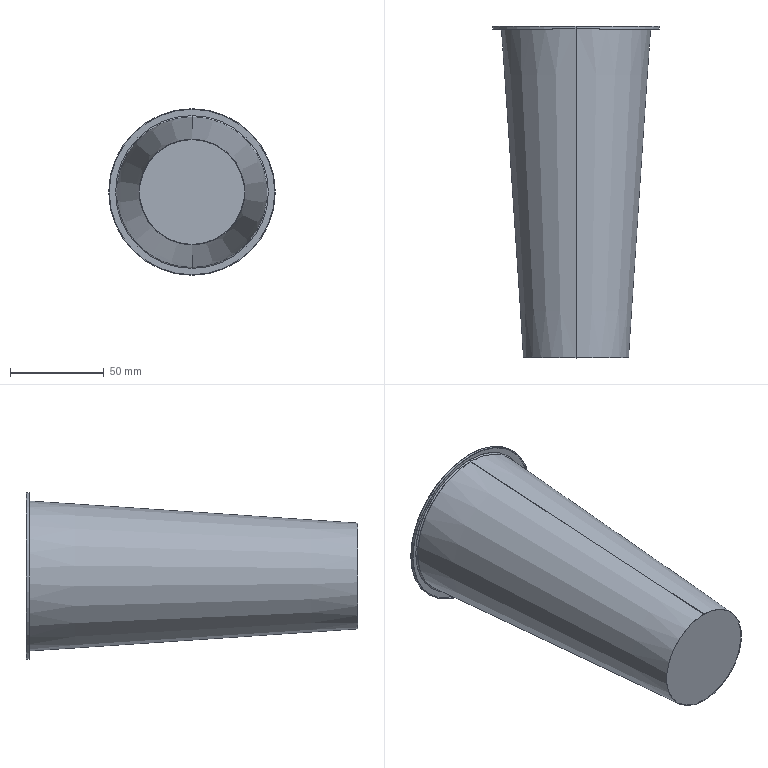Part | SolidWorks | features RefAxis 1, Revolution 1 | 1 solid | 19 faces | box 89 x 177.3 x 89 mm | volume 12581 mm3 | torus 6 | plane 5 | cone 4 | cylinder 4 | commonest cylinder face diameters 88.4 x2 89 x2
STEP:
#1=CARTESIAN_POINT('',(0.,-0.3,28.281));
#2=VERTEX_POINT('',#1);
#3=CARTESIAN_POINT('',(0.,-0.3,-28.281));
#4=VERTEX_POINT('',#3);
#5=CARTESIAN_POINT('',(0.,-0.3,0.));
#6=DIRECTION('',(0.,1.,0.));
#7=DIRECTION('',(0.,0.,1.));
#8=AXIS2_PLACEMENT_3D('',#5,#6,#7);
#9=CIRCLE('',#8,28.281);
#10=EDGE_CURVE('',#2,#4,#9,.T.);
#11=ORIENTED_EDGE('',*,*,#10,.T.);
#12=CARTESIAN_POINT('',(0.,176.047,-40.137));
#13=VERTEX_POINT('',#12);
#14=CARTESIAN_POINT('',(0.,176.047,-40.137));
#15=DIRECTION('',(0.,0.9977,-0.06708));
#16=VECTOR('',#15,1000.);
#17=LINE('',#14,#16);
#18=EDGE_CURVE('',#4,#13,#17,.T.);
#19=ORIENTED_EDGE('',*,*,#18,.T.);
#20=CARTESIAN_POINT('',(0.,176.047,40.137));
#21=VERTEX_POINT('',#20);
#22=CARTESIAN_POINT('',(0.,176.047,0.));
#23=DIRECTION('',(0.,1.,0.));
#24=DIRECTION('',(0.,0.,1.));
#25=AXIS2_PLACEMENT_3D('',#22,#23,#24);
#26=CIRCLE('',#25,40.137);
#27=EDGE_CURVE('',#21,#13,#26,.T.);
#28=ORIENTED_EDGE('',*,*,#27,.F.);
#29=CARTESIAN_POINT('',(0.,176.047,40.137));
#30=DIRECTION('',(0.,0.9977,0.06708));
#31=VECTOR('',#30,1000.);
#32=LINE('',#29,#31);
#33=EDGE_CURVE('',#2,#21,#32,.T.);
#34=ORIENTED_EDGE('',*,*,#33,.F.);
#35=EDGE_LOOP('',(#11,#19,#28,#34));
#36=FACE_OUTER_BOUND('',#35,.T.);
#37=CARTESIAN_POINT('',(0.,176.047,0.));
#38=DIRECTION('',(0.,1.,0.));
#39=DIRECTION('',(0.,0.,1.));
#40=AXIS2_PLACEMENT_3D('',#37,#38,#39);
#41=CONICAL_SURFACE('',#40,40.137,0.06713);
#42=ADVANCED_FACE('',(#36),#41,.T.);
#43=CARTESIAN_POINT('',(0.,176.7,-40.835));
#44=VERTEX_POINT('',#43);
#45=CARTESIAN_POINT('',(0.,176.7,40.835));
#46=VERTEX_POINT('',#45);
#47=CARTESIAN_POINT('',(0.,176.7,0.));
#48=DIRECTION('',(0.,1.,0.));
#49=DIRECTION('',(0.,0.,1.));
#50=AXIS2_PLACEMENT_3D('',#47,#48,#49);
#51=CIRCLE('',#50,40.835);
#52=EDGE_CURVE('',#44,#46,#51,.T.);
#53=ORIENTED_EDGE('',*,*,#52,.F.);
#54=CARTESIAN_POINT('',(0.,176.,-40.835));
#55=DIRECTION('',(1.,0.,0.));
#56=DIRECTION('',(0.,0.,-1.));
#57=AXIS2_PLACEMENT_3D('',#54,#55,#56);
#58=CIRCLE('',#57,0.7);
#59=EDGE_CURVE('',#44,#13,#58,.T.);
#60=ORIENTED_EDGE('',*,*,#59,.T.);
#61=CARTESIAN_POINT('',(0.,176.047,0.));
#62=DIRECTION('',(0.,1.,0.));
#63=DIRECTION('',(0.,0.,1.));
#64=AXIS2_PLACEMENT_3D('',#61,#62,#63);
#65=CIRCLE('',#64,40.137);
#66=EDGE_CURVE('',#13,#21,#65,.T.);
#67=ORIENTED_EDGE('',*,*,#66,.T.);
#68=CARTESIAN_POINT('',(0.,176.,40.835));
#69=DIRECTION('',(-1.,0.,0.));
#70=DIRECTION('',(0.,0.,1.));
#71=AXIS2_PLACEMENT_3D('',#68,#69,#70);
#72=CIRCLE('',#71,0.7);
#73=EDGE_CURVE('',#46,#21,#72,.T.);
#74=ORIENTED_EDGE('',*,*,#73,.F.);
#75=EDGE_LOOP('',(#53,#60,#67,#74));
#76=FACE_OUTER_BOUND('',#75,.T.);
#77=CARTESIAN_POINT('',(0.,176.,0.));
#78=DIRECTION('',(0.,1.,0.));
#79=DIRECTION('',(0.,0.,1.));
#80=AXIS2_PLACEMENT_3D('',#77,#78,#79);
#81=TOROIDAL_SURFACE('',#80,40.835,0.7);
#82=ADVANCED_FACE('',(#76),#81,.F.);
#83=CARTESIAN_POINT('',(0.,175.4,-44.2));
#84=VERTEX_POINT('',#83);
#85=CARTESIAN_POINT('',(0.,175.4,44.2));
#86=VERTEX_POINT('',#85);
#87=CARTESIAN_POINT('',(0.,175.4,0.));
#88=DIRECTION('',(0.,1.,0.));
#89=DIRECTION('',(0.,0.,1.));
#90=AXIS2_PLACEMENT_3D('',#87,#88,#89);
#91=CIRCLE('',#90,44.2);
#92=EDGE_CURVE('',#84,#86,#91,.T.);
#93=ORIENTED_EDGE('',*,*,#92,.F.);
#94=CARTESIAN_POINT('',(0.,176.7,-44.2));
#95=VERTEX_POINT('',#94);
#96=CARTESIAN_POINT('',(0.,0.,-44.2));
#97=DIRECTION('',(0.,1.,0.));
#98=VECTOR('',#97,1000.);
#99=LINE('',#96,#98);
#100=EDGE_CURVE('',#84,#95,#99,.T.);
#101=ORIENTED_EDGE('',*,*,#100,.T.);
#102=CARTESIAN_POINT('',(0.,176.7,44.2));
#103=VERTEX_POINT('',#102);
#104=CARTESIAN_POINT('',(0.,176.7,0.));
#105=DIRECTION('',(0.,1.,0.));
#106=DIRECTION('',(0.,0.,1.));
#107=AXIS2_PLACEMENT_3D('',#104,#105,#106);
#108=CIRCLE('',#107,44.2);
#109=EDGE_CURVE('',#95,#103,#108,.T.);
#110=ORIENTED_EDGE('',*,*,#109,.T.);
#111=CARTESIAN_POINT('',(0.,0.,44.2));
#112=DIRECTION('',(0.,1.,0.));
#113=VECTOR('',#112,1000.);
#114=LINE('',#111,#113);
#115=EDGE_CURVE('',#86,#103,#114,.T.);
#116=ORIENTED_EDGE('',*,*,#115,.F.);
#117=EDGE_LOOP('',(#93,#101,#110,#116));
#118=FACE_OUTER_BOUND('',#117,.T.);
#119=CARTESIAN_POINT('',(0.,0.,0.));
#120=DIRECTION('',(0.,1.,0.));
#121=DIRECTION('',(0.,0.,1.));
#122=AXIS2_PLACEMENT_3D('',#119,#120,#121);
#123=CYLINDRICAL_SURFACE('',#122,44.2);
#124=ADVANCED_FACE('',(#118),#123,.F.);
#125=CARTESIAN_POINT('',(0.,175.4,44.5));
#126=VERTEX_POINT('',#125);
#127=CARTESIAN_POINT('',(0.,175.4,-44.5));
#128=VERTEX_POINT('',#127);
#129=CARTESIAN_POINT('',(0.,175.4,0.));
#130=DIRECTION('',(0.,1.,0.));
#131=DIRECTION('',(0.,0.,1.));
#132=AXIS2_PLACEMENT_3D('',#129,#130,#131);
#133=CIRCLE('',#132,44.5);
#134=EDGE_CURVE('',#126,#128,#133,.T.);
#135=ORIENTED_EDGE('',*,*,#134,.T.);
#136=CARTESIAN_POINT('',(0.,176.7,-44.5));
#137=VERTEX_POINT('',#136);
#138=CARTESIAN_POINT('',(0.,0.,-44.5));
#139=DIRECTION('',(0.,1.,0.));
#140=VECTOR('',#139,1000.);
#141=LINE('',#138,#140);
#142=EDGE_CURVE('',#128,#137,#141,.T.);
#143=ORIENTED_EDGE('',*,*,#142,.T.);
#144=CARTESIAN_POINT('',(0.,176.7,44.5));
#145=VERTEX_POINT('',#144);
#146=CARTESIAN_POINT('',(0.,176.7,0.));
#147=DIRECTION('',(0.,1.,0.));
#148=DIRECTION('',(0.,0.,1.));
#149=AXIS2_PLACEMENT_3D('',#146,#147,#148);
#150=CIRCLE('',#149,44.5);
#151=EDGE_CURVE('',#145,#137,#150,.T.);
#152=ORIENTED_EDGE('',*,*,#151,.F.);
#153=CARTESIAN_POINT('',(0.,0.,44.5));
#154=DIRECTION('',(0.,1.,0.));
#155=VECTOR('',#154,1000.);
#156=LINE('',#153,#155);
#157=EDGE_CURVE('',#126,#145,#156,.T.);
#158=ORIENTED_EDGE('',*,*,#157,.F.);
#159=EDGE_LOOP('',(#135,#143,#152,#158));
#160=FACE_OUTER_BOUND('',#159,.T.);
#161=CARTESIAN_POINT('',(0.,0.,0.));
#162=DIRECTION('',(0.,1.,0.));
#163=DIRECTION('',(0.,0.,1.));
#164=AXIS2_PLACEMENT_3D('',#161,#162,#163);
#165=CYLINDRICAL_SURFACE('',#164,44.5);
#166=ADVANCED_FACE('',(#160),#165,.T.);
#167=ORIENTED_EDGE('',*,*,#151,.T.);
#168=CARTESIAN_POINT('',(0.,177.,-44.2));
#169=VERTEX_POINT('',#168);
#170=CARTESIAN_POINT('',(0.,176.7,-44.2));
#171=DIRECTION('',(1.,0.,0.));
#172=DIRECTION('',(0.,0.,-1.));
#173=AXIS2_PLACEMENT_3D('',#170,#171,#172);
#174=CIRCLE('',#173,0.3);
#175=EDGE_CURVE('',#137,#169,#174,.T.);
#176=ORIENTED_EDGE('',*,*,#175,.T.);
#177=CARTESIAN_POINT('',(0.,177.,44.2));
#178=VERTEX_POINT('',#177);
#179=CARTESIAN_POINT('',(0.,177.,0.));
#180=DIRECTION('',(0.,1.,0.));
#181=DIRECTION('',(0.,0.,1.));
#182=AXIS2_PLACEMENT_3D('',#179,#180,#181);
#183=CIRCLE('',#182,44.2);
#184=EDGE_CURVE('',#178,#169,#183,.T.);
#185=ORIENTED_EDGE('',*,*,#184,.F.);
#186=CARTESIAN_POINT('',(0.,176.7,44.2));
#187=DIRECTION('',(-1.,0.,0.));
#188=DIRECTION('',(0.,0.,1.));
#189=AXIS2_PLACEMENT_3D('',#186,#187,#188);
#190=CIRCLE('',#189,0.3);
#191=EDGE_CURVE('',#145,#178,#190,.T.);
#192=ORIENTED_EDGE('',*,*,#191,.F.);
#193=EDGE_LOOP('',(#167,#176,#185,#192));
#194=FACE_OUTER_BOUND('',#193,.T.);
#195=CARTESIAN_POINT('',(0.,176.7,0.));
#196=DIRECTION('',(0.,1.,0.));
#197=DIRECTION('',(0.,0.,1.));
#198=AXIS2_PLACEMENT_3D('',#195,#196,#197);
#199=TOROIDAL_SURFACE('',#198,44.2,0.3);
#200=ADVANCED_FACE('',(#194),#199,.T.);
#201=CARTESIAN_POINT('',(0.,177.,40.835));
#202=VERTEX_POINT('',#201);
#203=CARTESIAN_POINT('',(0.,177.,-40.835));
#204=VERTEX_POINT('',#203);
#205=CARTESIAN_POINT('',(0.,177.,0.));
#206=DIRECTION('',(0.,1.,0.));
#207=DIRECTION('',(0.,0.,1.));
#208=AXIS2_PLACEMENT_3D('',#205,#206,#207);
#209=CIRCLE('',#208,40.835);
#210=EDGE_CURVE('',#202,#204,#209,.T.);
#211=ORIENTED_EDGE('',*,*,#210,.T.);
#212=CARTESIAN_POINT('',(0.,176.067,-39.837));
#213=VERTEX_POINT('',#212);
#214=CARTESIAN_POINT('',(0.,176.,-40.835));
#215=DIRECTION('',(1.,0.,0.));
#216=DIRECTION('',(0.,0.,-1.));
#217=AXIS2_PLACEMENT_3D('',#214,#215,#216);
#218=CIRCLE('',#217,1.);
#219=EDGE_CURVE('',#204,#213,#218,.T.);
#220=ORIENTED_EDGE('',*,*,#219,.T.);
#221=CARTESIAN_POINT('',(0.,176.067,39.837));
#222=VERTEX_POINT('',#221);
#223=CARTESIAN_POINT('',(0.,176.067,0.));
#224=DIRECTION('',(0.,1.,0.));
#225=DIRECTION('',(0.,0.,1.));
#226=AXIS2_PLACEMENT_3D('',#223,#224,#225);
#227=CIRCLE('',#226,39.837);
#228=EDGE_CURVE('',#222,#213,#227,.T.);
#229=ORIENTED_EDGE('',*,*,#228,.F.);
#230=CARTESIAN_POINT('',(0.,176.,40.835));
#231=DIRECTION('',(-1.,0.,0.));
#232=DIRECTION('',(0.,0.,1.));
#233=AXIS2_PLACEMENT_3D('',#230,#231,#232);
#234=CIRCLE('',#233,1.);
#235=EDGE_CURVE('',#202,#222,#234,.T.);
#236=ORIENTED_EDGE('',*,*,#235,.F.);
#237=EDGE_LOOP('',(#211,#220,#229,#236));
#238=FACE_OUTER_BOUND('',#237,.T.);
#239=CARTESIAN_POINT('',(0.,176.,0.));
#240=DIRECTION('',(0.,1.,0.));
#241=DIRECTION('',(0.,0.,1.));
#242=AXIS2_PLACEMENT_3D('',#239,#240,#241);
#243=TOROIDAL_SURFACE('',#242,40.835,1.);
#244=ADVANCED_FACE('',(#238),#243,.T.);
#245=CARTESIAN_POINT('',(0.,0.,-28.));
#246=VERTEX_POINT('',#245);
#247=CARTESIAN_POINT('',(0.,0.,28.));
#248=VERTEX_POINT('',#247);
#249=CARTESIAN_POINT('',(0.,0.,0.));
#250=DIRECTION('',(0.,1.,0.));
#251=DIRECTION('',(0.,0.,1.));
#252=AXIS2_PLACEMENT_3D('',#249,#250,#251);
#253=CIRCLE('',#252,28.);
#254=EDGE_CURVE('',#246,#248,#253,.T.);
#255=ORIENTED_EDGE('',*,*,#254,.F.);
#256=CARTESIAN_POINT('',(0.,0.,-28.));
#257=DIRECTION('',(0.,0.9977,-0.06708));
#258=VECTOR('',#257,1000.);
#259=LINE('',#256,#258);
#260=EDGE_CURVE('',#246,#213,#259,.T.);
#261=ORIENTED_EDGE('',*,*,#260,.T.);
#262=CARTESIAN_POINT('',(0.,176.067,0.));
#263=DIRECTION('',(0.,1.,0.));
#264=DIRECTION('',(0.,0.,1.));
#265=AXIS2_PLACEMENT_3D('',#262,#263,#264);
#266=CIRCLE('',#265,39.837);
#267=EDGE_CURVE('',#213,#222,#266,.T.);
#268=ORIENTED_EDGE('',*,*,#267,.T.);
#269=CARTESIAN_POINT('',(0.,0.,28.));
#270=DIRECTION('',(0.,0.9977,0.06708));
#271=VECTOR('',#270,1000.);
#272=LINE('',#269,#271);
#273=EDGE_CURVE('',#248,#222,#272,.T.);
#274=ORIENTED_EDGE('',*,*,#273,.F.);
#275=EDGE_LOOP('',(#255,#261,#268,#274));
#276=FACE_OUTER_BOUND('',#275,.T.);
#277=CARTESIAN_POINT('',(0.,0.,0.));
#278=DIRECTION('',(0.,1.,0.));
#279=DIRECTION('',(0.,0.,1.));
#280=AXIS2_PLACEMENT_3D('',#277,#278,#279);
#281=CONICAL_SURFACE('',#280,28.,0.06713);
#282=ADVANCED_FACE('',(#276),#281,.F.);
#283=CARTESIAN_POINT('',(0.,0.,0.));
#284=DIRECTION('',(0.,1.,0.));
#285=DIRECTION('',(0.,0.,1.));
#286=AXIS2_PLACEMENT_3D('',#283,#284,#285);
#287=CIRCLE('',#286,28.);
#288=EDGE_CURVE('',#248,#246,#287,.T.);
#289=ORIENTED_EDGE('',*,*,#288,.T.);
#290=ORIENTED_EDGE('',*,*,#254,.T.);
#291=EDGE_LOOP('',(#289,#290));
#292=FACE_OUTER_BOUND('',#291,.T.);
#293=CARTESIAN_POINT('',(-28.,0.,0.));
#294=DIRECTION('',(0.,1.,0.));
#295=DIRECTION('',(0.,0.,1.));
#296=AXIS2_PLACEMENT_3D('',#293,#294,#295);
#297=PLANE('',#296);
#298=ADVANCED_FACE('',(#292),#297,.T.);
#299=ORIENTED_EDGE('',*,*,#260,.F.);
#300=ORIENTED_EDGE('',*,*,#288,.F.);
#301=ORIENTED_EDGE('',*,*,#273,.T.);
#302=ORIENTED_EDGE('',*,*,#228,.T.);
#303=EDGE_LOOP('',(#299,#300,#301,#302));
#304=FACE_OUTER_BOUND('',#303,.T.);
#305=CARTESIAN_POINT('',(0.,0.,0.));
#306=DIRECTION('',(0.,1.,0.));
#307=DIRECTION('',(0.,0.,1.));
#308=AXIS2_PLACEMENT_3D('',#305,#306,#307);
#309=CONICAL_SURFACE('',#308,28.,0.06713);
#310=ADVANCED_FACE('',(#304),#309,.F.);
#311=ORIENTED_EDGE('',*,*,#219,.F.);
#312=CARTESIAN_POINT('',(0.,177.,0.));
#313=DIRECTION('',(0.,1.,0.));
#314=DIRECTION('',(0.,0.,1.));
#315=AXIS2_PLACEMENT_3D('',#312,#313,#314);
#316=CIRCLE('',#315,40.835);
#317=EDGE_CURVE('',#204,#202,#316,.T.);
#318=ORIENTED_EDGE('',*,*,#317,.T.);
#319=ORIENTED_EDGE('',*,*,#235,.T.);
#320=ORIENTED_EDGE('',*,*,#267,.F.);
#321=EDGE_LOOP('',(#311,#318,#319,#320));
#322=FACE_OUTER_BOUND('',#321,.T.);
#323=CARTESIAN_POINT('',(0.,176.,0.));
#324=DIRECTION('',(0.,1.,0.));
#325=DIRECTION('',(0.,0.,1.));
#326=AXIS2_PLACEMENT_3D('',#323,#324,#325);
#327=TOROIDAL_SURFACE('',#326,40.835,1.);
#328=ADVANCED_FACE('',(#322),#327,.T.);
#329=ORIENTED_EDGE('',*,*,#184,.T.);
#330=CARTESIAN_POINT('',(0.,177.,0.));
#331=DIRECTION('',(0.,1.,0.));
#332=DIRECTION('',(0.,0.,1.));
#333=AXIS2_PLACEMENT_3D('',#330,#331,#332);
#334=CIRCLE('',#333,44.2);
#335=EDGE_CURVE('',#169,#178,#334,.T.);
#336=ORIENTED_EDGE('',*,*,#335,.T.);
#337=EDGE_LOOP('',(#329,#336));
#338=FACE_OUTER_BOUND('',#337,.T.);
#339=ORIENTED_EDGE('',*,*,#210,.F.);
#340=ORIENTED_EDGE('',*,*,#317,.F.);
#341=EDGE_LOOP('',(#339,#340));
#342=FACE_BOUND('',#341,.T.);
#343=CARTESIAN_POINT('',(-44.2,177.,0.));
#344=DIRECTION('',(0.,1.,0.));
#345=DIRECTION('',(0.,0.,1.));
#346=AXIS2_PLACEMENT_3D('',#343,#344,#345);
#347=PLANE('',#346);
#348=ADVANCED_FACE('',(#338,#342),#347,.T.);
#349=ORIENTED_EDGE('',*,*,#175,.F.);
#350=CARTESIAN_POINT('',(0.,176.7,0.));
#351=DIRECTION('',(0.,1.,0.));
#352=DIRECTION('',(0.,0.,1.));
#353=AXIS2_PLACEMENT_3D('',#350,#351,#352);
#354=CIRCLE('',#353,44.5);
#355=EDGE_CURVE('',#137,#145,#354,.T.);
#356=ORIENTED_EDGE('',*,*,#355,.T.);
#357=ORIENTED_EDGE('',*,*,#191,.T.);
#358=ORIENTED_EDGE('',*,*,#335,.F.);
#359=EDGE_LOOP('',(#349,#356,#357,#358));
#360=FACE_OUTER_BOUND('',#359,.T.);
#361=CARTESIAN_POINT('',(0.,176.7,0.));
#362=DIRECTION('',(0.,1.,0.));
#363=DIRECTION('',(0.,0.,1.));
#364=AXIS2_PLACEMENT_3D('',#361,#362,#363);
#365=TOROIDAL_SURFACE('',#364,44.2,0.3);
#366=ADVANCED_FACE('',(#360),#365,.T.);
#367=ORIENTED_EDGE('',*,*,#142,.F.);
#368=CARTESIAN_POINT('',(0.,175.4,0.));
#369=DIRECTION('',(0.,1.,0.));
#370=DIRECTION('',(0.,0.,1.));
#371=AXIS2_PLACEMENT_3D('',#368,#369,#370);
#372=CIRCLE('',#371,44.5);
#373=EDGE_CURVE('',#128,#126,#372,.T.);
#374=ORIENTED_EDGE('',*,*,#373,.T.);
#375=ORIENTED_EDGE('',*,*,#157,.T.);
#376=ORIENTED_EDGE('',*,*,#355,.F.);
#377=EDGE_LOOP('',(#367,#374,#375,#376));
#378=FACE_OUTER_BOUND('',#377,.T.);
#379=CARTESIAN_POINT('',(0.,0.,0.));
#380=DIRECTION('',(0.,1.,0.));
#381=DIRECTION('',(0.,0.,1.));
#382=AXIS2_PLACEMENT_3D('',#379,#380,#381);
#383=CYLINDRICAL_SURFACE('',#382,44.5);
#384=ADVANCED_FACE('',(#378),#383,.T.);
#385=CARTESIAN_POINT('',(0.,175.4,0.));
#386=DIRECTION('',(0.,1.,0.));
#387=DIRECTION('',(0.,0.,1.));
#388=AXIS2_PLACEMENT_3D('',#385,#386,#387);
#389=CIRCLE('',#388,44.2);
#390=EDGE_CURVE('',#86,#84,#389,.T.);
#391=ORIENTED_EDGE('',*,*,#390,.T.);
#392=ORIENTED_EDGE('',*,*,#92,.T.);
#393=EDGE_LOOP('',(#391,#392));
#394=FACE_BOUND('',#393,.T.);
#395=ORIENTED_EDGE('',*,*,#134,.F.);
#396=ORIENTED_EDGE('',*,*,#373,.F.);
#397=EDGE_LOOP('',(#395,#396));
#398=FACE_OUTER_BOUND('',#397,.T.);
#399=CARTESIAN_POINT('',(-44.5,175.4,0.));
#400=DIRECTION('',(0.,-1.,0.));
#401=DIRECTION('',(0.,0.,-1.));
#402=AXIS2_PLACEMENT_3D('',#399,#400,#401);
#403=PLANE('',#402);
#404=ADVANCED_FACE('',(#394,#398),#403,.T.);
#405=ORIENTED_EDGE('',*,*,#100,.F.);
#406=ORIENTED_EDGE('',*,*,#390,.F.);
#407=ORIENTED_EDGE('',*,*,#115,.T.);
#408=CARTESIAN_POINT('',(0.,176.7,0.));
#409=DIRECTION('',(0.,1.,0.));
#410=DIRECTION('',(0.,0.,1.));
#411=AXIS2_PLACEMENT_3D('',#408,#409,#410);
#412=CIRCLE('',#411,44.2);
#413=EDGE_CURVE('',#103,#95,#412,.T.);
#414=ORIENTED_EDGE('',*,*,#413,.T.);
#415=EDGE_LOOP('',(#405,#406,#407,#414));
#416=FACE_OUTER_BOUND('',#415,.T.);
#417=CARTESIAN_POINT('',(0.,0.,0.));
#418=DIRECTION('',(0.,1.,0.));
#419=DIRECTION('',(0.,0.,1.));
#420=AXIS2_PLACEMENT_3D('',#417,#418,#419);
#421=CYLINDRICAL_SURFACE('',#420,44.2);
#422=ADVANCED_FACE('',(#416),#421,.F.);
#423=CARTESIAN_POINT('',(0.,176.7,0.));
#424=DIRECTION('',(0.,1.,0.));
#425=DIRECTION('',(0.,0.,1.));
#426=AXIS2_PLACEMENT_3D('',#423,#424,#425);
#427=CIRCLE('',#426,40.835);
#428=EDGE_CURVE('',#46,#44,#427,.T.);
#429=ORIENTED_EDGE('',*,*,#428,.T.);
#430=ORIENTED_EDGE('',*,*,#52,.T.);
#431=EDGE_LOOP('',(#429,#430));
#432=FACE_BOUND('',#431,.T.);
#433=ORIENTED_EDGE('',*,*,#413,.F.);
#434=ORIENTED_EDGE('',*,*,#109,.F.);
#435=EDGE_LOOP('',(#433,#434));
#436=FACE_OUTER_BOUND('',#435,.T.);
#437=CARTESIAN_POINT('',(-44.2,176.7,0.));
#438=DIRECTION('',(0.,-1.,0.));
#439=DIRECTION('',(0.,0.,-1.));
#440=AXIS2_PLACEMENT_3D('',#437,#438,#439);
#441=PLANE('',#440);
#442=ADVANCED_FACE('',(#432,#436),#441,.T.);
#443=ORIENTED_EDGE('',*,*,#59,.F.);
#444=ORIENTED_EDGE('',*,*,#428,.F.);
#445=ORIENTED_EDGE('',*,*,#73,.T.);
#446=ORIENTED_EDGE('',*,*,#27,.T.);
#447=EDGE_LOOP('',(#443,#444,#445,#446));
#448=FACE_OUTER_BOUND('',#447,.T.);
#449=CARTESIAN_POINT('',(0.,176.,0.));
#450=DIRECTION('',(0.,1.,0.));
#451=DIRECTION('',(0.,0.,1.));
#452=AXIS2_PLACEMENT_3D('',#449,#450,#451);
#453=TOROIDAL_SURFACE('',#452,40.835,0.7);
#454=ADVANCED_FACE('',(#448),#453,.F.);
#455=ORIENTED_EDGE('',*,*,#18,.F.);
#456=CARTESIAN_POINT('',(0.,-0.3,0.));
#457=DIRECTION('',(0.,1.,0.));
#458=DIRECTION('',(0.,0.,1.));
#459=AXIS2_PLACEMENT_3D('',#456,#457,#458);
#460=CIRCLE('',#459,28.281);
#461=EDGE_CURVE('',#4,#2,#460,.T.);
#462=ORIENTED_EDGE('',*,*,#461,.T.);
#463=ORIENTED_EDGE('',*,*,#33,.T.);
#464=ORIENTED_EDGE('',*,*,#66,.F.);
#465=EDGE_LOOP('',(#455,#462,#463,#464));
#466=FACE_OUTER_BOUND('',#465,.T.);
#467=CARTESIAN_POINT('',(0.,176.047,0.));
#468=DIRECTION('',(0.,1.,0.));
#469=DIRECTION('',(0.,0.,1.));
#470=AXIS2_PLACEMENT_3D('',#467,#468,#469);
#471=CONICAL_SURFACE('',#470,40.137,0.06713);
#472=ADVANCED_FACE('',(#466),#471,.T.);
#473=ORIENTED_EDGE('',*,*,#10,.F.);
#474=ORIENTED_EDGE('',*,*,#461,.F.);
#475=EDGE_LOOP('',(#473,#474));
#476=FACE_OUTER_BOUND('',#475,.T.);
#477=CARTESIAN_POINT('',(-28.281,-0.3,0.));
#478=DIRECTION('',(0.,-1.,0.));
#479=DIRECTION('',(0.,0.,-1.));
#480=AXIS2_PLACEMENT_3D('',#477,#478,#479);
#481=PLANE('',#480);
#482=ADVANCED_FACE('',(#476),#481,.T.);
#483=CLOSED_SHELL('',(#42,#82,#124,#166,#200,#244,#282,#298,#310,#328,#348,#366,#384,#404,#422,#442,#454,#472,#482));
#484=MANIFOLD_SOLID_BREP('',#483);
#485=CARTESIAN_POINT('',(0.,0.,0.));
#486=DIRECTION('',(0.,0.,1.));
#487=DIRECTION('',(1.,0.,0.));
#488=AXIS2_PLACEMENT_3D('',#485,#486,#487);
#489=(LENGTH_UNIT()NAMED_UNIT(*)SI_UNIT(.MILLI.,.METRE.));
#490=UNCERTAINTY_MEASURE_WITH_UNIT(LENGTH_MEASURE(0.00001),#489,'','');
#491=(NAMED_UNIT(*)PLANE_ANGLE_UNIT()SI_UNIT($,.RADIAN.));
#492=(NAMED_UNIT(*)SI_UNIT($,.STERADIAN.)SOLID_ANGLE_UNIT());
#493=(GEOMETRIC_REPRESENTATION_CONTEXT(3)GLOBAL_UNCERTAINTY_ASSIGNED_CONTEXT((#490))GLOBAL_UNIT_ASSIGNED_CONTEXT((#489,#491,#492))REPRESENTATION_CONTEXT('',''));
#494=ADVANCED_BREP_SHAPE_REPRESENTATION('',(#484,#488),#493);